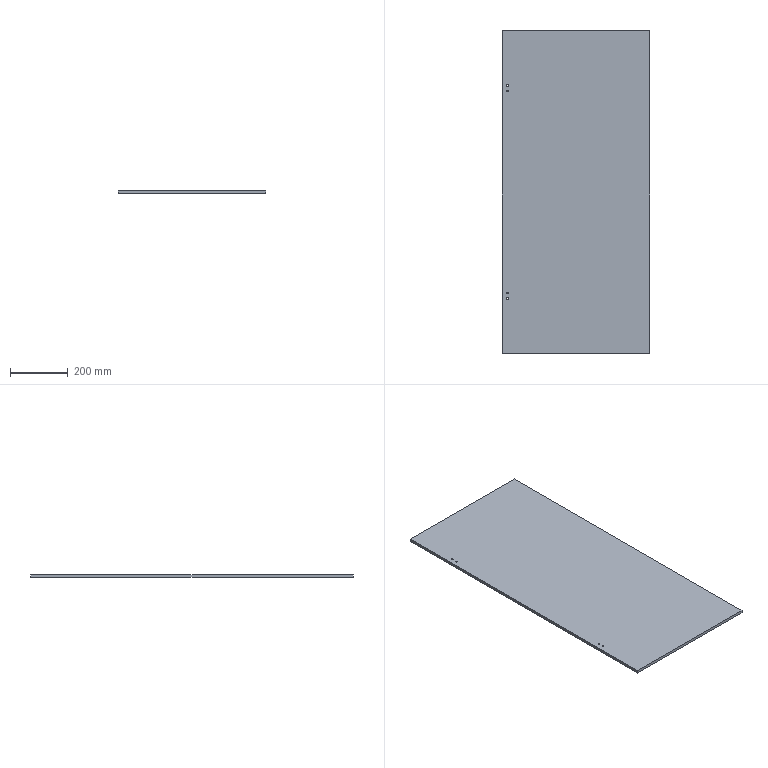Part | 1 solid | 14 faces | box 512 x 1121 x 10 mm | volume 5738389 mm3 | cylinder 8 | plane 6 | commonest cylinder face diameters 6 x8
STEP:
#1=CARTESIAN_POINT('',(-241.,370.5,-10.));
#2=VERTEX_POINT('',#1);
#3=CARTESIAN_POINT('',(-235.,370.5,-10.));
#4=VERTEX_POINT('',#3);
#5=CARTESIAN_POINT('',(-238.,370.5,-10.));
#6=DIRECTION('',(0.,0.,1.));
#7=DIRECTION('',(1.,0.,0.));
#8=AXIS2_PLACEMENT_3D('',#5,#6,#7);
#9=CIRCLE('',#8,3.);
#10=EDGE_CURVE('',#2,#4,#9,.T.);
#11=ORIENTED_EDGE('',*,*,#10,.F.);
#12=CARTESIAN_POINT('',(-241.,370.5,0.));
#13=VERTEX_POINT('',#12);
#14=CARTESIAN_POINT('',(-241.,370.5,-10.));
#15=DIRECTION('',(0.,0.,1.));
#16=VECTOR('',#15,1000.);
#17=LINE('',#14,#16);
#18=EDGE_CURVE('',#2,#13,#17,.T.);
#19=ORIENTED_EDGE('',*,*,#18,.T.);
#20=CARTESIAN_POINT('',(-235.,370.5,0.));
#21=VERTEX_POINT('',#20);
#22=CARTESIAN_POINT('',(-238.,370.5,0.));
#23=DIRECTION('',(0.,0.,1.));
#24=DIRECTION('',(1.,0.,0.));
#25=AXIS2_PLACEMENT_3D('',#22,#23,#24);
#26=CIRCLE('',#25,3.);
#27=EDGE_CURVE('',#13,#21,#26,.T.);
#28=ORIENTED_EDGE('',*,*,#27,.T.);
#29=CARTESIAN_POINT('',(-235.,370.5,-10.));
#30=DIRECTION('',(0.,0.,1.));
#31=VECTOR('',#30,1000.);
#32=LINE('',#29,#31);
#33=EDGE_CURVE('',#4,#21,#32,.T.);
#34=ORIENTED_EDGE('',*,*,#33,.F.);
#35=EDGE_LOOP('',(#11,#19,#28,#34));
#36=FACE_OUTER_BOUND('',#35,.T.);
#37=CARTESIAN_POINT('',(-238.,370.5,-10.));
#38=DIRECTION('',(0.,0.,1.));
#39=DIRECTION('',(1.,0.,0.));
#40=AXIS2_PLACEMENT_3D('',#37,#38,#39);
#41=CYLINDRICAL_SURFACE('',#40,3.);
#42=ADVANCED_FACE('',(#36),#41,.F.);
#43=CARTESIAN_POINT('',(-241.,351.5,-10.));
#44=VERTEX_POINT('',#43);
#45=CARTESIAN_POINT('',(-235.,351.5,-10.));
#46=VERTEX_POINT('',#45);
#47=CARTESIAN_POINT('',(-238.,351.5,-10.));
#48=DIRECTION('',(0.,0.,1.));
#49=DIRECTION('',(1.,0.,0.));
#50=AXIS2_PLACEMENT_3D('',#47,#48,#49);
#51=CIRCLE('',#50,3.);
#52=EDGE_CURVE('',#44,#46,#51,.T.);
#53=ORIENTED_EDGE('',*,*,#52,.F.);
#54=CARTESIAN_POINT('',(-241.,351.5,0.));
#55=VERTEX_POINT('',#54);
#56=CARTESIAN_POINT('',(-241.,351.5,-10.));
#57=DIRECTION('',(0.,0.,1.));
#58=VECTOR('',#57,1000.);
#59=LINE('',#56,#58);
#60=EDGE_CURVE('',#44,#55,#59,.T.);
#61=ORIENTED_EDGE('',*,*,#60,.T.);
#62=CARTESIAN_POINT('',(-235.,351.5,0.));
#63=VERTEX_POINT('',#62);
#64=CARTESIAN_POINT('',(-238.,351.5,0.));
#65=DIRECTION('',(0.,0.,1.));
#66=DIRECTION('',(1.,0.,0.));
#67=AXIS2_PLACEMENT_3D('',#64,#65,#66);
#68=CIRCLE('',#67,3.);
#69=EDGE_CURVE('',#55,#63,#68,.T.);
#70=ORIENTED_EDGE('',*,*,#69,.T.);
#71=CARTESIAN_POINT('',(-235.,351.5,-10.));
#72=DIRECTION('',(0.,0.,1.));
#73=VECTOR('',#72,1000.);
#74=LINE('',#71,#73);
#75=EDGE_CURVE('',#46,#63,#74,.T.);
#76=ORIENTED_EDGE('',*,*,#75,.F.);
#77=EDGE_LOOP('',(#53,#61,#70,#76));
#78=FACE_OUTER_BOUND('',#77,.T.);
#79=CARTESIAN_POINT('',(-238.,351.5,-10.));
#80=DIRECTION('',(0.,0.,1.));
#81=DIRECTION('',(1.,0.,0.));
#82=AXIS2_PLACEMENT_3D('',#79,#80,#81);
#83=CYLINDRICAL_SURFACE('',#82,3.);
#84=ADVANCED_FACE('',(#78),#83,.F.);
#85=CARTESIAN_POINT('',(-241.,-351.5,-10.));
#86=VERTEX_POINT('',#85);
#87=CARTESIAN_POINT('',(-235.,-351.5,-10.));
#88=VERTEX_POINT('',#87);
#89=CARTESIAN_POINT('',(-238.,-351.5,-10.));
#90=DIRECTION('',(0.,0.,1.));
#91=DIRECTION('',(-1.,0.,0.));
#92=AXIS2_PLACEMENT_3D('',#89,#90,#91);
#93=CIRCLE('',#92,3.);
#94=EDGE_CURVE('',#86,#88,#93,.T.);
#95=ORIENTED_EDGE('',*,*,#94,.F.);
#96=CARTESIAN_POINT('',(-241.,-351.5,0.));
#97=VERTEX_POINT('',#96);
#98=CARTESIAN_POINT('',(-241.,-351.5,-10.));
#99=DIRECTION('',(0.,0.,1.));
#100=VECTOR('',#99,1000.);
#101=LINE('',#98,#100);
#102=EDGE_CURVE('',#86,#97,#101,.T.);
#103=ORIENTED_EDGE('',*,*,#102,.T.);
#104=CARTESIAN_POINT('',(-235.,-351.5,0.));
#105=VERTEX_POINT('',#104);
#106=CARTESIAN_POINT('',(-238.,-351.5,0.));
#107=DIRECTION('',(0.,0.,1.));
#108=DIRECTION('',(-1.,0.,0.));
#109=AXIS2_PLACEMENT_3D('',#106,#107,#108);
#110=CIRCLE('',#109,3.);
#111=EDGE_CURVE('',#97,#105,#110,.T.);
#112=ORIENTED_EDGE('',*,*,#111,.T.);
#113=CARTESIAN_POINT('',(-235.,-351.5,-10.));
#114=DIRECTION('',(0.,0.,1.));
#115=VECTOR('',#114,1000.);
#116=LINE('',#113,#115);
#117=EDGE_CURVE('',#88,#105,#116,.T.);
#118=ORIENTED_EDGE('',*,*,#117,.F.);
#119=EDGE_LOOP('',(#95,#103,#112,#118));
#120=FACE_OUTER_BOUND('',#119,.T.);
#121=CARTESIAN_POINT('',(-238.,-351.5,-10.));
#122=DIRECTION('',(0.,0.,1.));
#123=DIRECTION('',(1.,0.,0.));
#124=AXIS2_PLACEMENT_3D('',#121,#122,#123);
#125=CYLINDRICAL_SURFACE('',#124,3.);
#126=ADVANCED_FACE('',(#120),#125,.F.);
#127=CARTESIAN_POINT('',(-241.,-370.5,-10.));
#128=VERTEX_POINT('',#127);
#129=CARTESIAN_POINT('',(-235.,-370.5,-10.));
#130=VERTEX_POINT('',#129);
#131=CARTESIAN_POINT('',(-238.,-370.5,-10.));
#132=DIRECTION('',(0.,0.,1.));
#133=DIRECTION('',(-1.,0.,0.));
#134=AXIS2_PLACEMENT_3D('',#131,#132,#133);
#135=CIRCLE('',#134,3.);
#136=EDGE_CURVE('',#128,#130,#135,.T.);
#137=ORIENTED_EDGE('',*,*,#136,.F.);
#138=CARTESIAN_POINT('',(-241.,-370.5,0.));
#139=VERTEX_POINT('',#138);
#140=CARTESIAN_POINT('',(-241.,-370.5,-10.));
#141=DIRECTION('',(0.,0.,1.));
#142=VECTOR('',#141,1000.);
#143=LINE('',#140,#142);
#144=EDGE_CURVE('',#128,#139,#143,.T.);
#145=ORIENTED_EDGE('',*,*,#144,.T.);
#146=CARTESIAN_POINT('',(-235.,-370.5,0.));
#147=VERTEX_POINT('',#146);
#148=CARTESIAN_POINT('',(-238.,-370.5,0.));
#149=DIRECTION('',(0.,0.,1.));
#150=DIRECTION('',(-1.,0.,0.));
#151=AXIS2_PLACEMENT_3D('',#148,#149,#150);
#152=CIRCLE('',#151,3.);
#153=EDGE_CURVE('',#139,#147,#152,.T.);
#154=ORIENTED_EDGE('',*,*,#153,.T.);
#155=CARTESIAN_POINT('',(-235.,-370.5,-10.));
#156=DIRECTION('',(0.,0.,1.));
#157=VECTOR('',#156,1000.);
#158=LINE('',#155,#157);
#159=EDGE_CURVE('',#130,#147,#158,.T.);
#160=ORIENTED_EDGE('',*,*,#159,.F.);
#161=EDGE_LOOP('',(#137,#145,#154,#160));
#162=FACE_OUTER_BOUND('',#161,.T.);
#163=CARTESIAN_POINT('',(-238.,-370.5,-10.));
#164=DIRECTION('',(0.,0.,1.));
#165=DIRECTION('',(1.,0.,0.));
#166=AXIS2_PLACEMENT_3D('',#163,#164,#165);
#167=CYLINDRICAL_SURFACE('',#166,3.);
#168=ADVANCED_FACE('',(#162),#167,.F.);
#169=CARTESIAN_POINT('',(256.,-560.5,0.));
#170=VERTEX_POINT('',#169);
#171=CARTESIAN_POINT('',(256.,560.5,0.));
#172=VERTEX_POINT('',#171);
#173=CARTESIAN_POINT('',(256.,560.5,0.));
#174=DIRECTION('',(0.,1.,0.));
#175=VECTOR('',#174,1000.);
#176=LINE('',#173,#175);
#177=EDGE_CURVE('',#170,#172,#176,.T.);
#178=ORIENTED_EDGE('',*,*,#177,.F.);
#179=CARTESIAN_POINT('',(256.,-560.5,-10.));
#180=VERTEX_POINT('',#179);
#181=CARTESIAN_POINT('',(256.,-560.5,-10.));
#182=DIRECTION('',(0.,0.,1.));
#183=VECTOR('',#182,1000.);
#184=LINE('',#181,#183);
#185=EDGE_CURVE('',#180,#170,#184,.T.);
#186=ORIENTED_EDGE('',*,*,#185,.F.);
#187=CARTESIAN_POINT('',(256.,560.5,-10.));
#188=VERTEX_POINT('',#187);
#189=CARTESIAN_POINT('',(256.,560.5,-10.));
#190=DIRECTION('',(0.,1.,0.));
#191=VECTOR('',#190,1000.);
#192=LINE('',#189,#191);
#193=EDGE_CURVE('',#180,#188,#192,.T.);
#194=ORIENTED_EDGE('',*,*,#193,.T.);
#195=CARTESIAN_POINT('',(256.,560.5,-10.));
#196=DIRECTION('',(0.,0.,1.));
#197=VECTOR('',#196,1000.);
#198=LINE('',#195,#197);
#199=EDGE_CURVE('',#188,#172,#198,.T.);
#200=ORIENTED_EDGE('',*,*,#199,.T.);
#201=EDGE_LOOP('',(#178,#186,#194,#200));
#202=FACE_OUTER_BOUND('',#201,.T.);
#203=CARTESIAN_POINT('',(256.,560.5,-10.));
#204=DIRECTION('',(1.,0.,0.));
#205=DIRECTION('',(0.,1.,0.));
#206=AXIS2_PLACEMENT_3D('',#203,#204,#205);
#207=PLANE('',#206);
#208=ADVANCED_FACE('',(#202),#207,.T.);
#209=CARTESIAN_POINT('',(-256.,-560.5,0.));
#210=VERTEX_POINT('',#209);
#211=CARTESIAN_POINT('',(-256.,-560.5,0.));
#212=DIRECTION('',(1.,0.,0.));
#213=VECTOR('',#212,1000.);
#214=LINE('',#211,#213);
#215=EDGE_CURVE('',#210,#170,#214,.T.);
#216=ORIENTED_EDGE('',*,*,#215,.F.);
#217=CARTESIAN_POINT('',(-256.,-560.5,-10.));
#218=VERTEX_POINT('',#217);
#219=CARTESIAN_POINT('',(-256.,-560.5,-10.));
#220=DIRECTION('',(0.,0.,1.));
#221=VECTOR('',#220,1000.);
#222=LINE('',#219,#221);
#223=EDGE_CURVE('',#218,#210,#222,.T.);
#224=ORIENTED_EDGE('',*,*,#223,.F.);
#225=CARTESIAN_POINT('',(-256.,-560.5,-10.));
#226=DIRECTION('',(1.,0.,0.));
#227=VECTOR('',#226,1000.);
#228=LINE('',#225,#227);
#229=EDGE_CURVE('',#218,#180,#228,.T.);
#230=ORIENTED_EDGE('',*,*,#229,.T.);
#231=ORIENTED_EDGE('',*,*,#185,.T.);
#232=EDGE_LOOP('',(#216,#224,#230,#231));
#233=FACE_OUTER_BOUND('',#232,.T.);
#234=CARTESIAN_POINT('',(-256.,-560.5,-10.));
#235=DIRECTION('',(0.,-1.,0.));
#236=DIRECTION('',(0.,0.,-1.));
#237=AXIS2_PLACEMENT_3D('',#234,#235,#236);
#238=PLANE('',#237);
#239=ADVANCED_FACE('',(#233),#238,.T.);
#240=CARTESIAN_POINT('',(-256.,560.5,0.));
#241=VERTEX_POINT('',#240);
#242=CARTESIAN_POINT('',(-256.,560.5,0.));
#243=DIRECTION('',(0.,-1.,0.));
#244=VECTOR('',#243,1000.);
#245=LINE('',#242,#244);
#246=EDGE_CURVE('',#241,#210,#245,.T.);
#247=ORIENTED_EDGE('',*,*,#246,.F.);
#248=CARTESIAN_POINT('',(-256.,560.5,-10.));
#249=VERTEX_POINT('',#248);
#250=CARTESIAN_POINT('',(-256.,560.5,-10.));
#251=DIRECTION('',(0.,0.,1.));
#252=VECTOR('',#251,1000.);
#253=LINE('',#250,#252);
#254=EDGE_CURVE('',#249,#241,#253,.T.);
#255=ORIENTED_EDGE('',*,*,#254,.F.);
#256=CARTESIAN_POINT('',(-256.,560.5,-10.));
#257=DIRECTION('',(0.,-1.,0.));
#258=VECTOR('',#257,1000.);
#259=LINE('',#256,#258);
#260=EDGE_CURVE('',#249,#218,#259,.T.);
#261=ORIENTED_EDGE('',*,*,#260,.T.);
#262=ORIENTED_EDGE('',*,*,#223,.T.);
#263=EDGE_LOOP('',(#247,#255,#261,#262));
#264=FACE_OUTER_BOUND('',#263,.T.);
#265=CARTESIAN_POINT('',(-256.,560.5,-10.));
#266=DIRECTION('',(-1.,0.,0.));
#267=DIRECTION('',(0.,-1.,0.));
#268=AXIS2_PLACEMENT_3D('',#265,#266,#267);
#269=PLANE('',#268);
#270=ADVANCED_FACE('',(#264),#269,.T.);
#271=CARTESIAN_POINT('',(-256.,560.5,0.));
#272=DIRECTION('',(-1.,0.,0.));
#273=VECTOR('',#272,1000.);
#274=LINE('',#271,#273);
#275=EDGE_CURVE('',#172,#241,#274,.T.);
#276=ORIENTED_EDGE('',*,*,#275,.F.);
#277=ORIENTED_EDGE('',*,*,#199,.F.);
#278=CARTESIAN_POINT('',(-256.,560.5,-10.));
#279=DIRECTION('',(-1.,0.,0.));
#280=VECTOR('',#279,1000.);
#281=LINE('',#278,#280);
#282=EDGE_CURVE('',#188,#249,#281,.T.);
#283=ORIENTED_EDGE('',*,*,#282,.T.);
#284=ORIENTED_EDGE('',*,*,#254,.T.);
#285=EDGE_LOOP('',(#276,#277,#283,#284));
#286=FACE_OUTER_BOUND('',#285,.T.);
#287=CARTESIAN_POINT('',(-256.,560.5,-10.));
#288=DIRECTION('',(0.,1.,0.));
#289=DIRECTION('',(0.,0.,1.));
#290=AXIS2_PLACEMENT_3D('',#287,#288,#289);
#291=PLANE('',#290);
#292=ADVANCED_FACE('',(#286),#291,.T.);
#293=CARTESIAN_POINT('',(-238.,370.5,-10.));
#294=DIRECTION('',(0.,0.,1.));
#295=DIRECTION('',(1.,0.,0.));
#296=AXIS2_PLACEMENT_3D('',#293,#294,#295);
#297=CIRCLE('',#296,3.);
#298=EDGE_CURVE('',#4,#2,#297,.T.);
#299=ORIENTED_EDGE('',*,*,#298,.T.);
#300=ORIENTED_EDGE('',*,*,#10,.T.);
#301=EDGE_LOOP('',(#299,#300));
#302=FACE_BOUND('',#301,.T.);
#303=CARTESIAN_POINT('',(-238.,351.5,-10.));
#304=DIRECTION('',(0.,0.,1.));
#305=DIRECTION('',(1.,0.,0.));
#306=AXIS2_PLACEMENT_3D('',#303,#304,#305);
#307=CIRCLE('',#306,3.);
#308=EDGE_CURVE('',#46,#44,#307,.T.);
#309=ORIENTED_EDGE('',*,*,#308,.T.);
#310=ORIENTED_EDGE('',*,*,#52,.T.);
#311=EDGE_LOOP('',(#309,#310));
#312=FACE_BOUND('',#311,.T.);
#313=CARTESIAN_POINT('',(-238.,-351.5,-10.));
#314=DIRECTION('',(0.,0.,1.));
#315=DIRECTION('',(-1.,0.,0.));
#316=AXIS2_PLACEMENT_3D('',#313,#314,#315);
#317=CIRCLE('',#316,3.);
#318=EDGE_CURVE('',#88,#86,#317,.T.);
#319=ORIENTED_EDGE('',*,*,#318,.T.);
#320=ORIENTED_EDGE('',*,*,#94,.T.);
#321=EDGE_LOOP('',(#319,#320));
#322=FACE_BOUND('',#321,.T.);
#323=CARTESIAN_POINT('',(-238.,-370.5,-10.));
#324=DIRECTION('',(0.,0.,1.));
#325=DIRECTION('',(-1.,0.,0.));
#326=AXIS2_PLACEMENT_3D('',#323,#324,#325);
#327=CIRCLE('',#326,3.);
#328=EDGE_CURVE('',#130,#128,#327,.T.);
#329=ORIENTED_EDGE('',*,*,#328,.T.);
#330=ORIENTED_EDGE('',*,*,#136,.T.);
#331=EDGE_LOOP('',(#329,#330));
#332=FACE_BOUND('',#331,.T.);
#333=ORIENTED_EDGE('',*,*,#193,.F.);
#334=ORIENTED_EDGE('',*,*,#229,.F.);
#335=ORIENTED_EDGE('',*,*,#260,.F.);
#336=ORIENTED_EDGE('',*,*,#282,.F.);
#337=EDGE_LOOP('',(#333,#334,#335,#336));
#338=FACE_OUTER_BOUND('',#337,.T.);
#339=CARTESIAN_POINT('',(0.,0.,-10.));
#340=DIRECTION('',(0.,0.,1.));
#341=DIRECTION('',(1.,0.,0.));
#342=AXIS2_PLACEMENT_3D('',#339,#340,#341);
#343=PLANE('',#342);
#344=ADVANCED_FACE('',(#302,#312,#322,#332,#338),#343,.F.);
#345=CARTESIAN_POINT('',(-238.,370.5,0.));
#346=DIRECTION('',(0.,0.,1.));
#347=DIRECTION('',(1.,0.,0.));
#348=AXIS2_PLACEMENT_3D('',#345,#346,#347);
#349=CIRCLE('',#348,3.);
#350=EDGE_CURVE('',#21,#13,#349,.T.);
#351=ORIENTED_EDGE('',*,*,#350,.F.);
#352=ORIENTED_EDGE('',*,*,#27,.F.);
#353=EDGE_LOOP('',(#351,#352));
#354=FACE_BOUND('',#353,.T.);
#355=CARTESIAN_POINT('',(-238.,351.5,0.));
#356=DIRECTION('',(0.,0.,1.));
#357=DIRECTION('',(1.,0.,0.));
#358=AXIS2_PLACEMENT_3D('',#355,#356,#357);
#359=CIRCLE('',#358,3.);
#360=EDGE_CURVE('',#63,#55,#359,.T.);
#361=ORIENTED_EDGE('',*,*,#360,.F.);
#362=ORIENTED_EDGE('',*,*,#69,.F.);
#363=EDGE_LOOP('',(#361,#362));
#364=FACE_BOUND('',#363,.T.);
#365=CARTESIAN_POINT('',(-238.,-351.5,0.));
#366=DIRECTION('',(0.,0.,1.));
#367=DIRECTION('',(-1.,0.,0.));
#368=AXIS2_PLACEMENT_3D('',#365,#366,#367);
#369=CIRCLE('',#368,3.);
#370=EDGE_CURVE('',#105,#97,#369,.T.);
#371=ORIENTED_EDGE('',*,*,#370,.F.);
#372=ORIENTED_EDGE('',*,*,#111,.F.);
#373=EDGE_LOOP('',(#371,#372));
#374=FACE_BOUND('',#373,.T.);
#375=CARTESIAN_POINT('',(-238.,-370.5,0.));
#376=DIRECTION('',(0.,0.,1.));
#377=DIRECTION('',(-1.,0.,0.));
#378=AXIS2_PLACEMENT_3D('',#375,#376,#377);
#379=CIRCLE('',#378,3.);
#380=EDGE_CURVE('',#147,#139,#379,.T.);
#381=ORIENTED_EDGE('',*,*,#380,.F.);
#382=ORIENTED_EDGE('',*,*,#153,.F.);
#383=EDGE_LOOP('',(#381,#382));
#384=FACE_BOUND('',#383,.T.);
#385=ORIENTED_EDGE('',*,*,#177,.T.);
#386=ORIENTED_EDGE('',*,*,#275,.T.);
#387=ORIENTED_EDGE('',*,*,#246,.T.);
#388=ORIENTED_EDGE('',*,*,#215,.T.);
#389=EDGE_LOOP('',(#385,#386,#387,#388));
#390=FACE_OUTER_BOUND('',#389,.T.);
#391=CARTESIAN_POINT('',(0.,0.,0.));
#392=DIRECTION('',(0.,0.,1.));
#393=DIRECTION('',(1.,0.,0.));
#394=AXIS2_PLACEMENT_3D('',#391,#392,#393);
#395=PLANE('',#394);
#396=ADVANCED_FACE('',(#354,#364,#374,#384,#390),#395,.T.);
#397=ORIENTED_EDGE('',*,*,#144,.F.);
#398=ORIENTED_EDGE('',*,*,#328,.F.);
#399=ORIENTED_EDGE('',*,*,#159,.T.);
#400=ORIENTED_EDGE('',*,*,#380,.T.);
#401=EDGE_LOOP('',(#397,#398,#399,#400));
#402=FACE_OUTER_BOUND('',#401,.T.);
#403=CARTESIAN_POINT('',(-238.,-370.5,-10.));
#404=DIRECTION('',(0.,0.,1.));
#405=DIRECTION('',(1.,0.,0.));
#406=AXIS2_PLACEMENT_3D('',#403,#404,#405);
#407=CYLINDRICAL_SURFACE('',#406,3.);
#408=ADVANCED_FACE('',(#402),#407,.F.);
#409=ORIENTED_EDGE('',*,*,#102,.F.);
#410=ORIENTED_EDGE('',*,*,#318,.F.);
#411=ORIENTED_EDGE('',*,*,#117,.T.);
#412=ORIENTED_EDGE('',*,*,#370,.T.);
#413=EDGE_LOOP('',(#409,#410,#411,#412));
#414=FACE_OUTER_BOUND('',#413,.T.);
#415=CARTESIAN_POINT('',(-238.,-351.5,-10.));
#416=DIRECTION('',(0.,0.,1.));
#417=DIRECTION('',(1.,0.,0.));
#418=AXIS2_PLACEMENT_3D('',#415,#416,#417);
#419=CYLINDRICAL_SURFACE('',#418,3.);
#420=ADVANCED_FACE('',(#414),#419,.F.);
#421=ORIENTED_EDGE('',*,*,#60,.F.);
#422=ORIENTED_EDGE('',*,*,#308,.F.);
#423=ORIENTED_EDGE('',*,*,#75,.T.);
#424=ORIENTED_EDGE('',*,*,#360,.T.);
#425=EDGE_LOOP('',(#421,#422,#423,#424));
#426=FACE_OUTER_BOUND('',#425,.T.);
#427=CARTESIAN_POINT('',(-238.,351.5,-10.));
#428=DIRECTION('',(0.,0.,1.));
#429=DIRECTION('',(1.,0.,0.));
#430=AXIS2_PLACEMENT_3D('',#427,#428,#429);
#431=CYLINDRICAL_SURFACE('',#430,3.);
#432=ADVANCED_FACE('',(#426),#431,.F.);
#433=ORIENTED_EDGE('',*,*,#18,.F.);
#434=ORIENTED_EDGE('',*,*,#298,.F.);
#435=ORIENTED_EDGE('',*,*,#33,.T.);
#436=ORIENTED_EDGE('',*,*,#350,.T.);
#437=EDGE_LOOP('',(#433,#434,#435,#436));
#438=FACE_OUTER_BOUND('',#437,.T.);
#439=CARTESIAN_POINT('',(-238.,370.5,-10.));
#440=DIRECTION('',(0.,0.,1.));
#441=DIRECTION('',(1.,0.,0.));
#442=AXIS2_PLACEMENT_3D('',#439,#440,#441);
#443=CYLINDRICAL_SURFACE('',#442,3.);
#444=ADVANCED_FACE('',(#438),#443,.F.);
#445=CLOSED_SHELL('',(#42,#84,#126,#168,#208,#239,#270,#292,#344,#396,#408,#420,#432,#444));
#446=MANIFOLD_SOLID_BREP('',#445);
#447=CARTESIAN_POINT('',(0.,0.,0.));
#448=DIRECTION('',(0.,0.,1.));
#449=DIRECTION('',(1.,0.,0.));
#450=AXIS2_PLACEMENT_3D('',#447,#448,#449);
#451=(LENGTH_UNIT()NAMED_UNIT(*)SI_UNIT(.MILLI.,.METRE.));
#452=UNCERTAINTY_MEASURE_WITH_UNIT(LENGTH_MEASURE(0.00001),#451,'','');
#453=(NAMED_UNIT(*)PLANE_ANGLE_UNIT()SI_UNIT($,.RADIAN.));
#454=(NAMED_UNIT(*)SI_UNIT($,.STERADIAN.)SOLID_ANGLE_UNIT());
#455=(GEOMETRIC_REPRESENTATION_CONTEXT(3)GLOBAL_UNCERTAINTY_ASSIGNED_CONTEXT((#452))GLOBAL_UNIT_ASSIGNED_CONTEXT((#451,#453,#454))REPRESENTATION_CONTEXT('',''));
#456=ADVANCED_BREP_SHAPE_REPRESENTATION('',(#446,#450),#455);